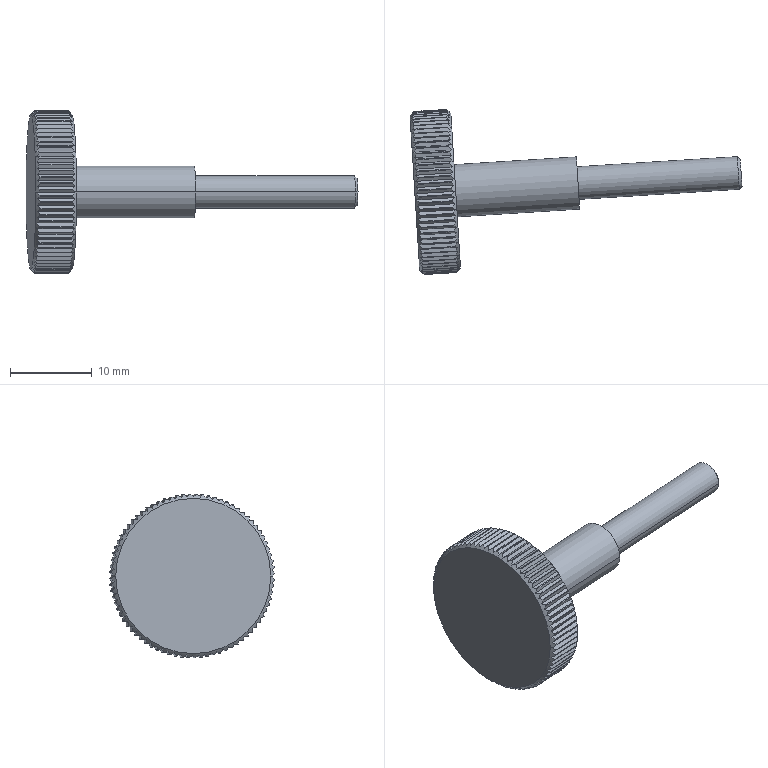Part | SolidWorks | features BaseBody 1 | 1 solid | 254 faces | box 40.621 x 20.205 x 19.993 mm | volume 2253 mm3 | plane 164 | cylinder 84 | cone 6 | commonest cylinder face diameters 20 x80 4 x2 6.4 x2